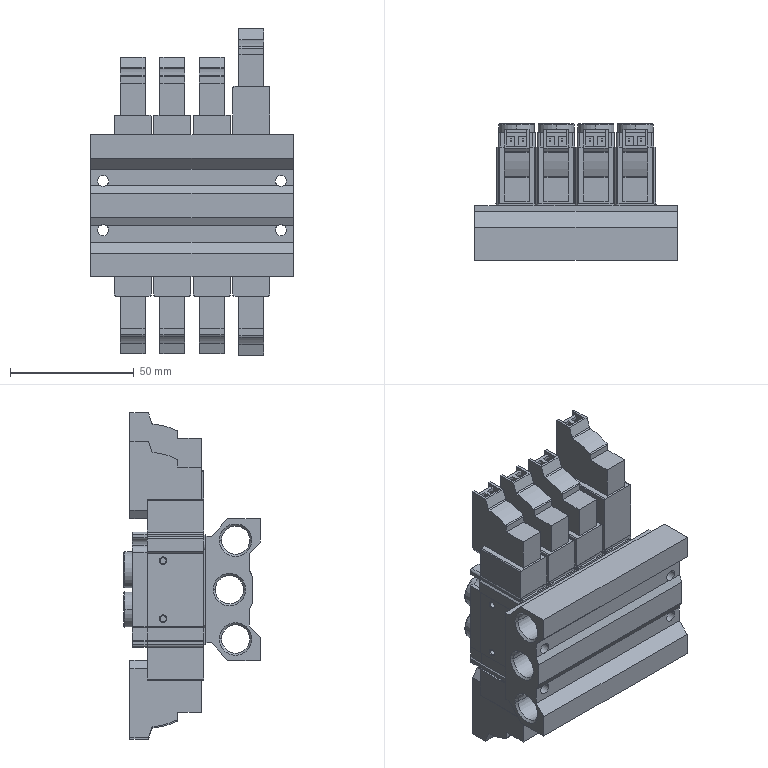Part | SolidWorks | 5 solids | 1052 faces | box 82 x 55.3 x 132 mm | volume 207310 mm3 | plane 646 | cylinder 306 | cone 84 | torus 16 | commonest cylinder face diameters 8.566 x40 2 x32 2.459 x32 0.8 x16 1 x16 1.2 x16